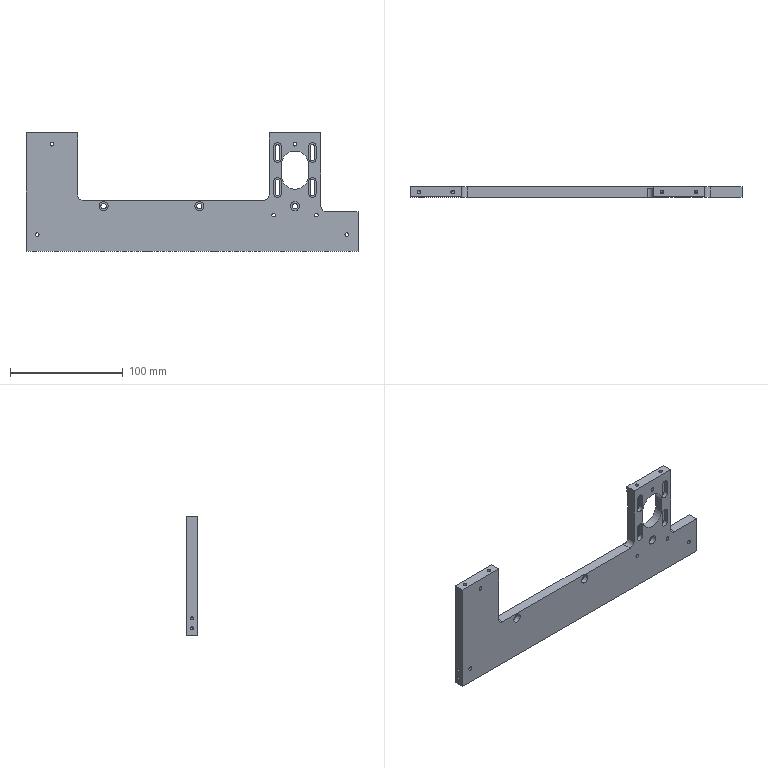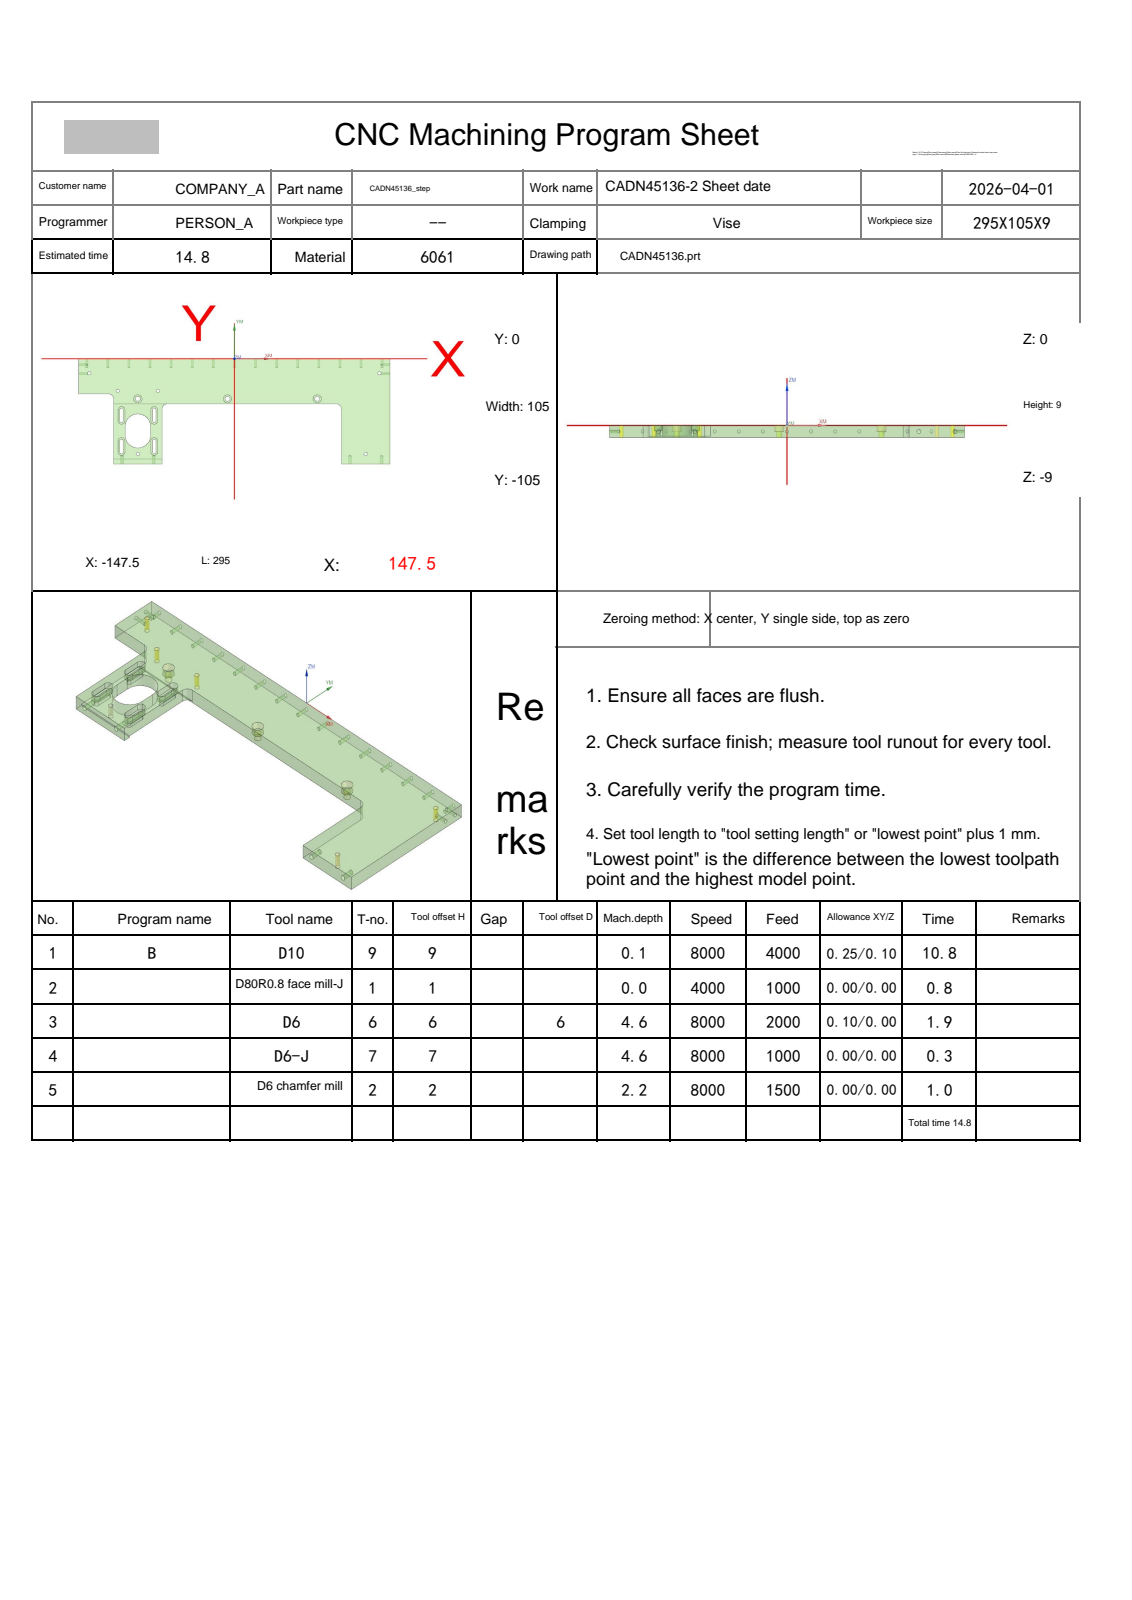NC program | NX | posted by the shop | part box 295 x 9 x 105 mm
Lines 2214 to 3343 of 3343:
N2 T01 M06
(D80R0.8 face mill-J  D=80. R=0.8 H=01 ce=0.00 di=0.00)
G00 G90 G54 X-199.499 Y-24.001 M03 S4000
G43 H01 Z20.
M08
Z2.
G01 Z0.0 F1000.
X-187.499
X179.503
G02 X187.499 Y-31.997 I-.004 J-8.
G01 Y-65.639
G02 X179.499 Y-73.639 I-8. J0.0
G01 X-187.499
X-199.499
Z2.
G00 Z20.
G91 G28 Z0.0
M05
M09
G91 G28 Z0.0
M01
N3 T06 M06
(D6  D=6. R=0. H=06 ce=0.10 di=0.00)
G00 G90 G54 X-91.5 Y-40. M03 S8000
G43 H06 Z20.
M08
Z.3
G41 D06
G01 X-91.505 Y-39.9 F2000.
G03 X-91.947 Y-39.547 I-.442 J-.1
X-92.4 Y-40. I0.0 J-.453
X-92.4 Y-40. Z-.05 I.9 J0.0
X-92.4 Y-40. Z-.4 I.9 J0.0
X-92.4 Y-40. Z-.75 I.9 J0.0
X-92.4 Y-40. Z-1.1 I.9 J0.0
X-92.4 Y-40. Z-1.45 I.9 J0.0
X-92.4 Y-40. Z-1.8 I.9 J0.0
X-92.4 Y-40. Z-2.15 I.9 J0.0
X-92.4 Y-40. Z-2.5 I.9 J0.0
X-92.4 Y-40. Z-2.85 I.9 J0.0
X-92.4 Y-40. Z-3.2 I.9 J0.0
X-92.4 Y-40. Z-3.55 I.9 J0.0
X-92.4 Y-40. Z-3.9 I.9 J0.0
X-92.4 Y-40. Z-4.25 I.9 J0.0
X-92.4 Y-40. Z-4.6 I.9 J0.0
X-91.5 Y-40.9 I.9 J0.0
X-90.6 Y-40. I0.0 J.9
X-91.5 Y-39.1 I-.9 J0.0
X-92.4 Y-40. I0.0 J-.9
X-91.947 Y-40.453 I.453 J0.0
X-91.505 Y-40.1 I0.0 J.453
G01 G40 X-91.5 Y-40.
G00 Z20.
X-6.5
Z.3
G41 D06
G01 X-6.505 Y-39.9
G03 X-6.947 Y-39.547 I-.442 J-.1
X-7.4 Y-40. I0.0 J-.453
X-7.4 Y-40. Z-.05 I.9 J0.0
X-7.4 Y-40. Z-.4 I.9 J0.0
X-7.4 Y-40. Z-.75 I.9 J0.0
X-7.4 Y-40. Z-1.1 I.9 J0.0
X-7.4 Y-40. Z-1.45 I.9 J0.0
X-7.4 Y-40. Z-1.8 I.9 J0.0
X-7.4 Y-40. Z-2.15 I.9 J0.0
X-7.4 Y-40. Z-2.5 I.9 J0.0
X-7.4 Y-40. Z-2.85 I.9 J0.0
X-7.4 Y-40. Z-3.2 I.9 J0.0
X-7.4 Y-40. Z-3.55 I.9 J0.0
X-7.4 Y-40. Z-3.9 I.9 J0.0
X-7.4 Y-40. Z-4.25 I.9 J0.0
X-7.4 Y-40. Z-4.6 I.9 J0.0
X-6.5 Y-40.9 I.9 J0.0
X-5.6 Y-40. I0.0 J.9
X-6.5 Y-39.1 I-.9 J0.0
X-7.4 Y-40. I0.0 J-.9
X-6.947 Y-40.453 I.453 J0.0
X-6.505 Y-40.1 I0.0 J.453
G01 G40 X-6.5 Y-40.
G00 Z20.
X78.5
Z.3
G41 D06
G01 X78.495 Y-39.9
G03 X78.053 Y-39.547 I-.442 J-.1
X77.6 Y-40. I0.0 J-.453
X77.6 Y-40. Z-.05 I.9 J0.0
X77.6 Y-40. Z-.4 I.9 J0.0
X77.6 Y-40. Z-.75 I.9 J0.0
X77.6 Y-40. Z-1.1 I.9 J0.0
X77.6 Y-40. Z-1.45 I.9 J0.0
X77.6 Y-40. Z-1.8 I.9 J0.0
X77.6 Y-40. Z-2.15 I.9 J0.0
X77.6 Y-40. Z-2.5 I.9 J0.0
X77.6 Y-40. Z-2.85 I.9 J0.0
X77.6 Y-40. Z-3.2 I.9 J0.0
X77.6 Y-40. Z-3.55 I.9 J0.0
X77.6 Y-40. Z-3.9 I.9 J0.0
X77.6 Y-40. Z-4.25 I.9 J0.0
X77.6 Y-40. Z-4.6 I.9 J0.0
X78.5 Y-40.9 I.9 J0.0
X79.4 Y-40. I0.0 J.9
X78.5 Y-39.1 I-.9 J0.0
X77.6 Y-40. I0.0 J-.9
X78.053 Y-40.453 I.453 J0.0
X78.495 Y-40.1 I0.0 J.453
G01 G40 X78.5 Y-40.
G00 Z20.
G00 G90 X-75.85 Y-57.849 M03 S8000
Z20.
Z1.
G01 Y-50.851 Z.633 F1200.
X-75.901 Y-50.8 Z.629
X-76. Z.624
X-76.099 Z.619
X-76.15 Y-50.851 Z.615
Y-62.149 Z.023
X-76.099 Y-62.2 Z.019
X-76. Z.014
X-75.901 Z.009
X-75.85 Y-62.149 Z.005
Y-62.05 Z0.0
Y-50.95 Z-.094
G03 X-76. Y-50.8 Z-.096 I-.15 J0.0
X-76.15 Y-50.95 Z-.098 I0.0 J-.15
G01 Y-62.05 Z-.191
G03 X-76. Y-62.2 Z-.193 I.15 J0.0
X-75.85 Y-62.05 Z-.195 I0.0 J.15
G01 Y-50.95 Z-.289
G03 X-76. Y-50.8 Z-.291 I-.15 J0.0
X-76.15 Y-50.95 Z-.293 I0.0 J-.15
G01 Y-62.05 Z-.386
G03 X-76. Y-62.2 Z-.388 I.15 J0.0
X-75.85 Y-62.05 Z-.39 I0.0 J.15
G01 Y-50.95 Z-.484
G03 X-76. Y-50.8 Z-.486 I-.15 J0.0
X-76.15 Y-50.95 Z-.488 I0.0 J-.15
G01 Y-62.05 Z-.581
G03 X-76. Y-62.2 Z-.583 I.15 J0.0
X-75.85 Y-62.05 Z-.585 I0.0 J.15
G01 Y-50.95 Z-.679
G03 X-76. Y-50.8 Z-.681 I-.15 J0.0
X-76.15 Y-50.95 Z-.683 I0.0 J-.15
G01 Y-62.05 Z-.776
G03 X-76. Y-62.2 Z-.778 I.15 J0.0
X-75.85 Y-62.05 Z-.78 I0.0 J.15
G01 Y-50.95 Z-.874
G03 X-76. Y-50.8 Z-.876 I-.15 J0.0
X-76.15 Y-50.95 Z-.878 I0.0 J-.15
G01 Y-62.05 Z-.971
G03 X-76. Y-62.2 Z-.973 I.15 J0.0
X-75.85 Y-62.05 Z-.975 I0.0 J.15
G01 Y-50.95 Z-1.069
G03 X-76. Y-50.8 Z-1.071 I-.15 J0.0
X-76.15 Y-50.95 Z-1.073 I0.0 J-.15
G01 Y-62.05 Z-1.166
G03 X-76. Y-62.2 Z-1.168 I.15 J0.0
X-75.85 Y-62.05 Z-1.17 I0.0 J.15
G01 Y-50.95 Z-1.264
G03 X-76. Y-50.8 Z-1.266 I-.15 J0.0
X-76.15 Y-50.95 Z-1.268 I0.0 J-.15
G01 Y-62.05 Z-1.361
G03 X-76. Y-62.2 Z-1.363 I.15 J0.0
X-75.85 Y-62.05 Z-1.365 I0.0 J.15
G01 Y-50.95 Z-1.459
G03 X-76. Y-50.8 Z-1.461 I-.15 J0.0
X-76.15 Y-50.95 Z-1.463 I0.0 J-.15
G01 Y-62.05 Z-1.556
G03 X-76. Y-62.2 Z-1.558 I.15 J0.0
X-75.85 Y-62.05 Z-1.56 I0.0 J.15
G01 Y-50.95 Z-1.654
G03 X-76. Y-50.8 Z-1.656 I-.15 J0.0
X-76.15 Y-50.95 Z-1.658 I0.0 J-.15
G01 Y-62.05 Z-1.751
G03 X-76. Y-62.2 Z-1.753 I.15 J0.0
X-75.85 Y-62.05 Z-1.755 I0.0 J.15
G01 Y-50.95 Z-1.849
G03 X-76. Y-50.8 Z-1.851 I-.15 J0.0
X-76.15 Y-50.95 Z-1.853 I0.0 J-.15
G01 Y-62.05 Z-1.946
G03 X-76. Y-62.2 Z-1.948 I.15 J0.0
X-75.85 Y-62.05 Z-1.95 I0.0 J.15
G01 Y-50.95 Z-2.044
G03 X-76. Y-50.8 Z-2.046 I-.15 J0.0
X-76.15 Y-50.95 Z-2.048 I0.0 J-.15
G01 Y-62.05 Z-2.141
G03 X-76. Y-62.2 Z-2.143 I.15 J0.0
X-75.85 Y-62.05 Z-2.145 I0.0 J.15
G01 Y-50.95 Z-2.239
G03 X-76. Y-50.8 Z-2.241 I-.15 J0.0
X-76.15 Y-50.95 Z-2.243 I0.0 J-.15
G01 Y-62.05 Z-2.336
G03 X-76. Y-62.2 Z-2.338 I.15 J0.0
X-75.85 Y-62.05 Z-2.34 I0.0 J.15
G01 Y-50.95 Z-2.434
G03 X-76. Y-50.8 Z-2.436 I-.15 J0.0
X-76.15 Y-50.95 Z-2.438 I0.0 J-.15
G01 Y-62.05 Z-2.531
G03 X-76. Y-62.2 Z-2.533 I.15 J0.0
X-75.85 Y-62.05 Z-2.535 I0.0 J.15
G01 Y-50.95 Z-2.629
G03 X-76. Y-50.8 Z-2.631 I-.15 J0.0
X-76.15 Y-50.95 Z-2.633 I0.0 J-.15
G01 Y-62.05 Z-2.726
G03 X-76. Y-62.2 Z-2.728 I.15 J0.0
X-75.85 Y-62.05 Z-2.73 I0.0 J.15
G01 Y-50.95 Z-2.824
G03 X-76. Y-50.8 Z-2.826 I-.15 J0.0
X-76.15 Y-50.95 Z-2.828 I0.0 J-.15
G01 Y-62.05 Z-2.921
G03 X-76. Y-62.2 Z-2.923 I.15 J0.0
X-75.85 Y-62.05 Z-2.925 I0.0 J.15
G01 Y-50.95 Z-3.019
G03 X-76. Y-50.8 Z-3.021 I-.15 J0.0
X-76.15 Y-50.95 Z-3.023 I0.0 J-.15
G01 Y-62.05 Z-3.116
G03 X-76. Y-62.2 Z-3.118 I.15 J0.0
X-75.85 Y-62.05 Z-3.12 I0.0 J.15
G01 Y-50.95 Z-3.214
G03 X-76. Y-50.8 Z-3.216 I-.15 J0.0
X-76.15 Y-50.95 Z-3.218 I0.0 J-.15
G01 Y-62.05 Z-3.311
G03 X-76. Y-62.2 Z-3.313 I.15 J0.0
X-75.85 Y-62.05 Z-3.315 I0.0 J.15
G01 Y-50.95 Z-3.409
G03 X-76. Y-50.8 Z-3.411 I-.15 J0.0
X-76.15 Y-50.95 Z-3.413 I0.0 J-.15
G01 Y-62.05 Z-3.506
G03 X-76. Y-62.2 Z-3.508 I.15 J0.0
X-75.85 Y-62.05 Z-3.51 I0.0 J.15
G01 Y-50.95 Z-3.604
G03 X-76. Y-50.8 Z-3.606 I-.15 J0.0
X-76.15 Y-50.95 Z-3.608 I0.0 J-.15
G01 Y-62.05 Z-3.701
G03 X-76. Y-62.2 Z-3.703 I.15 J0.0
X-75.85 Y-62.05 Z-3.705 I0.0 J.15
G01 Y-50.95 Z-3.799
G03 X-76. Y-50.8 Z-3.801 I-.15 J0.0
X-76.15 Y-50.95 Z-3.803 I0.0 J-.15
G01 Y-62.05 Z-3.896
G03 X-76. Y-62.2 Z-3.898 I.15 J0.0
X-75.85 Y-62.05 Z-3.9 I0.0 J.15
G01 Y-50.95
G03 X-76. Y-50.8 I-.15 J0.0
X-76.15 Y-50.95 I0.0 J-.15
G01 Y-62.05
G03 X-76. Y-62.2 I.15 J0.0
X-75.85 Y-62.05 I0.0 J.15
G01 Y-61.65
Z-2.9
G00 Z20.
X-106.85 Y-57.849
Z1.
G01 Y-50.851 Z.633
X-106.901 Y-50.8 Z.629
X-107.099 Z.619
X-107.15 Y-50.851 Z.615
Y-62.149 Z.023
X-107.099 Y-62.2 Z.019
X-106.901 Z.009
X-106.85 Y-62.149 Z.005
Y-62.05 Z0.0
Y-50.95 Z-.094
G03 X-107. Y-50.8 Z-.096 I-.15 J0.0
X-107.15 Y-50.95 Z-.098 I0.0 J-.15
G01 Y-62.05 Z-.191
G03 X-107. Y-62.2 Z-.193 I.15 J0.0
X-106.85 Y-62.05 Z-.195 I0.0 J.15
G01 Y-50.95 Z-.289
G03 X-107. Y-50.8 Z-.291 I-.15 J0.0
X-107.15 Y-50.95 Z-.293 I0.0 J-.15
G01 Y-62.05 Z-.386
G03 X-107. Y-62.2 Z-.388 I.15 J0.0
X-106.85 Y-62.05 Z-.39 I0.0 J.15
G01 Y-50.95 Z-.484
G03 X-107. Y-50.8 Z-.486 I-.15 J0.0
X-107.15 Y-50.95 Z-.488 I0.0 J-.15
G01 Y-62.05 Z-.581
G03 X-107. Y-62.2 Z-.583 I.15 J0.0
X-106.85 Y-62.05 Z-.585 I0.0 J.15
G01 Y-50.95 Z-.679
G03 X-107. Y-50.8 Z-.681 I-.15 J0.0
X-107.15 Y-50.95 Z-.683 I0.0 J-.15
G01 Y-62.05 Z-.776
G03 X-107. Y-62.2 Z-.778 I.15 J0.0
X-106.85 Y-62.05 Z-.78 I0.0 J.15
G01 Y-50.95 Z-.874
G03 X-107. Y-50.8 Z-.876 I-.15 J0.0
X-107.15 Y-50.95 Z-.878 I0.0 J-.15
G01 Y-62.05 Z-.971
G03 X-107. Y-62.2 Z-.973 I.15 J0.0
X-106.85 Y-62.05 Z-.975 I0.0 J.15
G01 Y-50.95 Z-1.069
G03 X-107. Y-50.8 Z-1.071 I-.15 J0.0
X-107.15 Y-50.95 Z-1.073 I0.0 J-.15
G01 Y-62.05 Z-1.166
G03 X-107. Y-62.2 Z-1.168 I.15 J0.0
X-106.85 Y-62.05 Z-1.17 I0.0 J.15
G01 Y-50.95 Z-1.264
G03 X-107. Y-50.8 Z-1.266 I-.15 J0.0
X-107.15 Y-50.95 Z-1.268 I0.0 J-.15
G01 Y-62.05 Z-1.361
G03 X-107. Y-62.2 Z-1.363 I.15 J0.0
X-106.85 Y-62.05 Z-1.365 I0.0 J.15
G01 Y-50.95 Z-1.459
G03 X-107. Y-50.8 Z-1.461 I-.15 J0.0
X-107.15 Y-50.95 Z-1.463 I0.0 J-.15
G01 Y-62.05 Z-1.556
G03 X-107. Y-62.2 Z-1.558 I.15 J0.0
X-106.85 Y-62.05 Z-1.56 I0.0 J.15
G01 Y-50.95 Z-1.654
G03 X-107. Y-50.8 Z-1.656 I-.15 J0.0
X-107.15 Y-50.95 Z-1.658 I0.0 J-.15
G01 Y-62.05 Z-1.751
G03 X-107. Y-62.2 Z-1.753 I.15 J0.0
X-106.85 Y-62.05 Z-1.755 I0.0 J.15
G01 Y-50.95 Z-1.849
G03 X-107. Y-50.8 Z-1.851 I-.15 J0.0
X-107.15 Y-50.95 Z-1.853 I0.0 J-.15
G01 Y-62.05 Z-1.946
G03 X-107. Y-62.2 Z-1.948 I.15 J0.0
X-106.85 Y-62.05 Z-1.95 I0.0 J.15
G01 Y-50.95 Z-2.044
G03 X-107. Y-50.8 Z-2.046 I-.15 J0.0
X-107.15 Y-50.95 Z-2.048 I0.0 J-.15
G01 Y-62.05 Z-2.141
G03 X-107. Y-62.2 Z-2.143 I.15 J0.0
X-106.85 Y-62.05 Z-2.145 I0.0 J.15
G01 Y-50.95 Z-2.239
G03 X-107. Y-50.8 Z-2.241 I-.15 J0.0
X-107.15 Y-50.95 Z-2.243 I0.0 J-.15
G01 Y-62.05 Z-2.336
G03 X-107. Y-62.2 Z-2.338 I.15 J0.0
X-106.85 Y-62.05 Z-2.34 I0.0 J.15
G01 Y-50.95 Z-2.434
G03 X-107. Y-50.8 Z-2.436 I-.15 J0.0
X-107.15 Y-50.95 Z-2.438 I0.0 J-.15
G01 Y-62.05 Z-2.531
G03 X-107. Y-62.2 Z-2.533 I.15 J0.0
X-106.85 Y-62.05 Z-2.535 I0.0 J.15
G01 Y-50.95 Z-2.629
G03 X-107. Y-50.8 Z-2.631 I-.15 J0.0
X-107.15 Y-50.95 Z-2.633 I0.0 J-.15
G01 Y-62.05 Z-2.726
G03 X-107. Y-62.2 Z-2.728 I.15 J0.0
X-106.85 Y-62.05 Z-2.73 I0.0 J.15
G01 Y-50.95 Z-2.824
G03 X-107. Y-50.8 Z-2.826 I-.15 J0.0
X-107.15 Y-50.95 Z-2.828 I0.0 J-.15
G01 Y-62.05 Z-2.921
G03 X-107. Y-62.2 Z-2.923 I.15 J0.0
X-106.85 Y-62.05 Z-2.925 I0.0 J.15
G01 Y-50.95 Z-3.019
G03 X-107. Y-50.8 Z-3.021 I-.15 J0.0
X-107.15 Y-50.95 Z-3.023 I0.0 J-.15
G01 Y-62.05 Z-3.116
G03 X-107. Y-62.2 Z-3.118 I.15 J0.0
X-106.85 Y-62.05 Z-3.12 I0.0 J.15
G01 Y-50.95 Z-3.214
G03 X-107. Y-50.8 Z-3.216 I-.15 J0.0
X-107.15 Y-50.95 Z-3.218 I0.0 J-.15
G01 Y-62.05 Z-3.311
G03 X-107. Y-62.2 Z-3.313 I.15 J0.0
X-106.85 Y-62.05 Z-3.315 I0.0 J.15
G01 Y-50.95 Z-3.409
G03 X-107. Y-50.8 Z-3.411 I-.15 J0.0
X-107.15 Y-50.95 Z-3.413 I0.0 J-.15
G01 Y-62.05 Z-3.506
G03 X-107. Y-62.2 Z-3.508 I.15 J0.0
X-106.85 Y-62.05 Z-3.51 I0.0 J.15
G01 Y-50.95 Z-3.604
G03 X-107. Y-50.8 Z-3.606 I-.15 J0.0
X-107.15 Y-50.95 Z-3.608 I0.0 J-.15
G01 Y-62.05 Z-3.701
G03 X-107. Y-62.2 Z-3.703 I.15 J0.0
X-106.85 Y-62.05 Z-3.705 I0.0 J.15
G01 Y-50.95 Z-3.799
G03 X-107. Y-50.8 Z-3.801 I-.15 J0.0
X-107.15 Y-50.95 Z-3.803 I0.0 J-.15
G01 Y-62.05 Z-3.896
G03 X-107. Y-62.2 Z-3.898 I.15 J0.0
X-106.85 Y-62.05 Z-3.9 I0.0 J.15
G01 Y-50.95
G03 X-107. Y-50.8 I-.15 J0.0
X-107.15 Y-50.95 I0.0 J-.15
G01 Y-62.05
G03 X-107. Y-62.2 I.15 J0.0
X-106.85 Y-62.05 I0.0 J.15
G01 Y-61.65
Z-2.9
G00 Z20.
Y-88.849
Z1.
G01 Y-81.95 Z.638
Y-81.851 Z.633
X-106.901 Y-81.8 Z.629
X-107. Z.624
X-107.099 Z.619
X-107.15 Y-81.851 Z.615
Y-93.149 Z.023
X-107.099 Y-93.2 Z.019
X-106.901 Z.009
X-106.85 Y-93.149 Z.005
Y-93.05 Z0.0
Y-81.95 Z-.094
G03 X-107. Y-81.8 Z-.096 I-.15 J0.0
X-107.15 Y-81.95 Z-.098 I0.0 J-.15
G01 Y-93.05 Z-.191
G03 X-107. Y-93.2 Z-.193 I.15 J0.0
X-106.85 Y-93.05 Z-.195 I0.0 J.15
G01 Y-81.95 Z-.289
G03 X-107. Y-81.8 Z-.291 I-.15 J0.0
X-107.15 Y-81.95 Z-.293 I0.0 J-.15
G01 Y-93.05 Z-.386
G03 X-107. Y-93.2 Z-.388 I.15 J0.0
X-106.85 Y-93.05 Z-.39 I0.0 J.15
G01 Y-81.95 Z-.484
G03 X-107. Y-81.8 Z-.486 I-.15 J0.0
X-107.15 Y-81.95 Z-.488 I0.0 J-.15
G01 Y-93.05 Z-.581
G03 X-107. Y-93.2 Z-.583 I.15 J0.0
X-106.85 Y-93.05 Z-.585 I0.0 J.15
G01 Y-81.95 Z-.679
G03 X-107. Y-81.8 Z-.681 I-.15 J0.0
X-107.15 Y-81.95 Z-.683 I0.0 J-.15
G01 Y-93.05 Z-.776
G03 X-107. Y-93.2 Z-.778 I.15 J0.0
X-106.85 Y-93.05 Z-.78 I0.0 J.15
G01 Y-81.95 Z-.874
G03 X-107. Y-81.8 Z-.876 I-.15 J0.0
X-107.15 Y-81.95 Z-.878 I0.0 J-.15
G01 Y-93.05 Z-.971
G03 X-107. Y-93.2 Z-.973 I.15 J0.0
X-106.85 Y-93.05 Z-.975 I0.0 J.15
G01 Y-81.95 Z-1.069
G03 X-107. Y-81.8 Z-1.071 I-.15 J0.0
X-107.15 Y-81.95 Z-1.073 I0.0 J-.15
G01 Y-93.05 Z-1.166
G03 X-107. Y-93.2 Z-1.168 I.15 J0.0
X-106.85 Y-93.05 Z-1.17 I0.0 J.15
G01 Y-81.95 Z-1.264
G03 X-107. Y-81.8 Z-1.266 I-.15 J0.0
X-107.15 Y-81.95 Z-1.268 I0.0 J-.15
G01 Y-93.05 Z-1.361
G03 X-107. Y-93.2 Z-1.363 I.15 J0.0
X-106.85 Y-93.05 Z-1.365 I0.0 J.15
G01 Y-81.95 Z-1.459
G03 X-107. Y-81.8 Z-1.461 I-.15 J0.0
X-107.15 Y-81.95 Z-1.463 I0.0 J-.15
G01 Y-93.05 Z-1.556
G03 X-107. Y-93.2 Z-1.558 I.15 J0.0
X-106.85 Y-93.05 Z-1.56 I0.0 J.15
G01 Y-81.95 Z-1.654
G03 X-107. Y-81.8 Z-1.656 I-.15 J0.0
X-107.15 Y-81.95 Z-1.658 I0.0 J-.15
G01 Y-93.05 Z-1.751
G03 X-107. Y-93.2 Z-1.753 I.15 J0.0
X-106.85 Y-93.05 Z-1.755 I0.0 J.15
G01 Y-81.95 Z-1.849
G03 X-107. Y-81.8 Z-1.851 I-.15 J0.0
X-107.15 Y-81.95 Z-1.853 I0.0 J-.15
G01 Y-93.05 Z-1.946
G03 X-107. Y-93.2 Z-1.948 I.15 J0.0
X-106.85 Y-93.05 Z-1.95 I0.0 J.15
G01 Y-81.95 Z-2.044
G03 X-107. Y-81.8 Z-2.046 I-.15 J0.0
X-107.15 Y-81.95 Z-2.048 I0.0 J-.15
G01 Y-93.05 Z-2.141
G03 X-107. Y-93.2 Z-2.143 I.15 J0.0
X-106.85 Y-93.05 Z-2.145 I0.0 J.15
G01 Y-81.95 Z-2.239
G03 X-107. Y-81.8 Z-2.241 I-.15 J0.0
X-107.15 Y-81.95 Z-2.243 I0.0 J-.15
G01 Y-93.05 Z-2.336
G03 X-107. Y-93.2 Z-2.338 I.15 J0.0
X-106.85 Y-93.05 Z-2.34 I0.0 J.15
G01 Y-81.95 Z-2.434
G03 X-107. Y-81.8 Z-2.436 I-.15 J0.0
X-107.15 Y-81.95 Z-2.438 I0.0 J-.15
G01 Y-93.05 Z-2.531
G03 X-107. Y-93.2 Z-2.533 I.15 J0.0
X-106.85 Y-93.05 Z-2.535 I0.0 J.15
G01 Y-81.95 Z-2.629
G03 X-107. Y-81.8 Z-2.631 I-.15 J0.0
X-107.15 Y-81.95 Z-2.633 I0.0 J-.15
G01 Y-93.05 Z-2.726
G03 X-107. Y-93.2 Z-2.728 I.15 J0.0
X-106.85 Y-93.05 Z-2.73 I0.0 J.15
G01 Y-81.95 Z-2.824
G03 X-107. Y-81.8 Z-2.826 I-.15 J0.0
X-107.15 Y-81.95 Z-2.828 I0.0 J-.15
G01 Y-93.05 Z-2.921
G03 X-107. Y-93.2 Z-2.923 I.15 J0.0
X-106.85 Y-93.05 Z-2.925 I0.0 J.15
G01 Y-81.95 Z-3.019
G03 X-107. Y-81.8 Z-3.021 I-.15 J0.0
X-107.15 Y-81.95 Z-3.023 I0.0 J-.15
G01 Y-93.05 Z-3.116
G03 X-107. Y-93.2 Z-3.118 I.15 J0.0
X-106.85 Y-93.05 Z-3.12 I0.0 J.15
G01 Y-81.95 Z-3.214
G03 X-107. Y-81.8 Z-3.216 I-.15 J0.0
X-107.15 Y-81.95 Z-3.218 I0.0 J-.15
G01 Y-93.05 Z-3.311
G03 X-107. Y-93.2 Z-3.313 I.15 J0.0
X-106.85 Y-93.05 Z-3.315 I0.0 J.15
G01 Y-81.95 Z-3.409
G03 X-107. Y-81.8 Z-3.411 I-.15 J0.0
X-107.15 Y-81.95 Z-3.413 I0.0 J-.15
G01 Y-93.05 Z-3.506
G03 X-107. Y-93.2 Z-3.508 I.15 J0.0
X-106.85 Y-93.05 Z-3.51 I0.0 J.15
G01 Y-81.95 Z-3.604
G03 X-107. Y-81.8 Z-3.606 I-.15 J0.0
X-107.15 Y-81.95 Z-3.608 I0.0 J-.15
G01 Y-93.05 Z-3.701
G03 X-107. Y-93.2 Z-3.703 I.15 J0.0
X-106.85 Y-93.05 Z-3.705 I0.0 J.15
G01 Y-81.95 Z-3.799
G03 X-107. Y-81.8 Z-3.801 I-.15 J0.0
X-107.15 Y-81.95 Z-3.803 I0.0 J-.15
G01 Y-93.05 Z-3.896
G03 X-107. Y-93.2 Z-3.898 I.15 J0.0
X-106.85 Y-93.05 Z-3.9 I0.0 J.15
G01 Y-81.95
G03 X-107. Y-81.8 I-.15 J0.0
X-107.15 Y-81.95 I0.0 J-.15
G01 Y-93.05
G03 X-107. Y-93.2 I.15 J0.0
X-106.85 Y-93.05 I0.0 J.15
G01 Y-92.65
Z-2.9
G00 Z20.
X-76.15 Y-86.151
Z1.
G01 Y-93.05 Z.638
Y-93.149 Z.633
X-76.099 Y-93.2 Z.629
X-75.901 Z.619
X-75.85 Y-93.149 Z.615
Y-81.851 Z.023
X-75.901 Y-81.8 Z.019
X-76. Z.014
X-76.099 Z.009
X-76.15 Y-81.851 Z.005
Y-81.95 Z0.0
Y-93.05 Z-.094
G03 X-76. Y-93.2 Z-.096 I.15 J0.0
X-75.85 Y-93.05 Z-.098 I0.0 J.15
G01 Y-81.95 Z-.191
G03 X-76. Y-81.8 Z-.193 I-.15 J0.0
X-76.15 Y-81.95 Z-.195 I0.0 J-.15
G01 Y-93.05 Z-.289
G03 X-76. Y-93.2 Z-.291 I.15 J0.0
X-75.85 Y-93.05 Z-.293 I0.0 J.15
G01 Y-81.95 Z-.386
G03 X-76. Y-81.8 Z-.388 I-.15 J0.0
X-76.15 Y-81.95 Z-.39 I0.0 J-.15
G01 Y-93.05 Z-.484
G03 X-76. Y-93.2 Z-.486 I.15 J0.0
X-75.85 Y-93.05 Z-.488 I0.0 J.15
G01 Y-81.95 Z-.581
G03 X-76. Y-81.8 Z-.583 I-.15 J0.0
X-76.15 Y-81.95 Z-.585 I0.0 J-.15
G01 Y-93.05 Z-.679
G03 X-76. Y-93.2 Z-.681 I.15 J0.0
X-75.85 Y-93.05 Z-.683 I0.0 J.15
G01 Y-81.95 Z-.776
G03 X-76. Y-81.8 Z-.778 I-.15 J0.0
X-76.15 Y-81.95 Z-.78 I0.0 J-.15
G01 Y-93.05 Z-.874
G03 X-76. Y-93.2 Z-.876 I.15 J0.0
X-75.85 Y-93.05 Z-.878 I0.0 J.15
G01 Y-81.95 Z-.971
G03 X-76. Y-81.8 Z-.973 I-.15 J0.0
X-76.15 Y-81.95 Z-.975 I0.0 J-.15
G01 Y-93.05 Z-1.069
G03 X-76. Y-93.2 Z-1.071 I.15 J0.0
X-75.85 Y-93.05 Z-1.073 I0.0 J.15
G01 Y-81.95 Z-1.166
G03 X-76. Y-81.8 Z-1.168 I-.15 J0.0
X-76.15 Y-81.95 Z-1.17 I0.0 J-.15
G01 Y-93.05 Z-1.264
G03 X-76. Y-93.2 Z-1.266 I.15 J0.0
X-75.85 Y-93.05 Z-1.268 I0.0 J.15
G01 Y-81.95 Z-1.361
G03 X-76. Y-81.8 Z-1.363 I-.15 J0.0
X-76.15 Y-81.95 Z-1.365 I0.0 J-.15
G01 Y-93.05 Z-1.459
G03 X-76. Y-93.2 Z-1.461 I.15 J0.0
X-75.85 Y-93.05 Z-1.463 I0.0 J.15
G01 Y-81.95 Z-1.556
G03 X-76. Y-81.8 Z-1.558 I-.15 J0.0
X-76.15 Y-81.95 Z-1.56 I0.0 J-.15
G01 Y-93.05 Z-1.654
G03 X-76. Y-93.2 Z-1.656 I.15 J0.0
X-75.85 Y-93.05 Z-1.658 I0.0 J.15
G01 Y-81.95 Z-1.751
G03 X-76. Y-81.8 Z-1.753 I-.15 J0.0
X-76.15 Y-81.95 Z-1.755 I0.0 J-.15
G01 Y-93.05 Z-1.849
G03 X-76. Y-93.2 Z-1.851 I.15 J0.0
X-75.85 Y-93.05 Z-1.853 I0.0 J.15
G01 Y-81.95 Z-1.946
G03 X-76. Y-81.8 Z-1.948 I-.15 J0.0
X-76.15 Y-81.95 Z-1.95 I0.0 J-.15
G01 Y-93.05 Z-2.044
G03 X-76. Y-93.2 Z-2.046 I.15 J0.0
X-75.85 Y-93.05 Z-2.048 I0.0 J.15
G01 Y-81.95 Z-2.141
G03 X-76. Y-81.8 Z-2.143 I-.15 J0.0
X-76.15 Y-81.95 Z-2.145 I0.0 J-.15
G01 Y-93.05 Z-2.239
G03 X-76. Y-93.2 Z-2.241 I.15 J0.0
X-75.85 Y-93.05 Z-2.243 I0.0 J.15
G01 Y-81.95 Z-2.336
G03 X-76. Y-81.8 Z-2.338 I-.15 J0.0
X-76.15 Y-81.95 Z-2.34 I0.0 J-.15
G01 Y-93.05 Z-2.434
G03 X-76. Y-93.2 Z-2.436 I.15 J0.0
X-75.85 Y-93.05 Z-2.438 I0.0 J.15
G01 Y-81.95 Z-2.531
G03 X-76. Y-81.8 Z-2.533 I-.15 J0.0
X-76.15 Y-81.95 Z-2.535 I0.0 J-.15
G01 Y-93.05 Z-2.629
G03 X-76. Y-93.2 Z-2.631 I.15 J0.0
X-75.85 Y-93.05 Z-2.633 I0.0 J.15
G01 Y-81.95 Z-2.726
G03 X-76. Y-81.8 Z-2.728 I-.15 J0.0
X-76.15 Y-81.95 Z-2.73 I0.0 J-.15
G01 Y-93.05 Z-2.824
G03 X-76. Y-93.2 Z-2.826 I.15 J0.0
X-75.85 Y-93.05 Z-2.828 I0.0 J.15
G01 Y-81.95 Z-2.921
G03 X-76. Y-81.8 Z-2.923 I-.15 J0.0
X-76.15 Y-81.95 Z-2.925 I0.0 J-.15
G01 Y-93.05 Z-3.019
G03 X-76. Y-93.2 Z-3.021 I.15 J0.0
X-75.85 Y-93.05 Z-3.023 I0.0 J.15
G01 Y-81.95 Z-3.116
G03 X-76. Y-81.8 Z-3.118 I-.15 J0.0
X-76.15 Y-81.95 Z-3.12 I0.0 J-.15
G01 Y-93.05 Z-3.214
G03 X-76. Y-93.2 Z-3.216 I.15 J0.0
X-75.85 Y-93.05 Z-3.218 I0.0 J.15
G01 Y-81.95 Z-3.311
G03 X-76. Y-81.8 Z-3.313 I-.15 J0.0
X-76.15 Y-81.95 Z-3.315 I0.0 J-.15
G01 Y-93.05 Z-3.409
G03 X-76. Y-93.2 Z-3.411 I.15 J0.0
X-75.85 Y-93.05 Z-3.413 I0.0 J.15
G01 Y-81.95 Z-3.506
G03 X-76. Y-81.8 Z-3.508 I-.15 J0.0
X-76.15 Y-81.95 Z-3.51 I0.0 J-.15
G01 Y-93.05 Z-3.604
G03 X-76. Y-93.2 Z-3.606 I.15 J0.0
X-75.85 Y-93.05 Z-3.608 I0.0 J.15
G01 Y-81.95 Z-3.701
G03 X-76. Y-81.8 Z-3.703 I-.15 J0.0
X-76.15 Y-81.95 Z-3.705 I0.0 J-.15
G01 Y-93.05 Z-3.799
G03 X-76. Y-93.2 Z-3.801 I.15 J0.0
X-75.85 Y-93.05 Z-3.803 I0.0 J.15
G01 Y-81.95 Z-3.896
G03 X-76. Y-81.8 Z-3.898 I-.15 J0.0
X-76.15 Y-81.95 Z-3.9 I0.0 J-.15
G01 Y-93.05
G03 X-76. Y-93.2 I.15 J0.0
X-75.85 Y-93.05 I0.0 J.15
G01 Y-81.95
G03 X-76. Y-81.8 I-.15 J0.0
X-76.15 Y-81.95 I0.0 J-.15
G01 Y-82.35
Z-2.9
G00 Z20.
G91 G28 Z0.0
M05
M09
G91 G28 Z0.0
M01
N4 T07 M06
(D6-J  D=6. R=0. H=07 ce=0.00 di=0.00)
G00 G90 G54 X-91.5 Y-40. M03 S8000
G43 H07 Z20.
M08
Z-4.6
G01 X-92.029 Y-39.718 F600.
X-92.18 Y-39.68
G03 X-92.5 Y-40. I0.0 J-.32
X-91.5 Y-41. I1. J0.0
X-90.5 Y-40. I0.0 J1.
X-91.5 Y-39. I-1. J0.0
X-92.5 Y-40. I0.0 J-1.
X-92.378 Y-40.479 I1. J0.0
X-92.097 Y-40.646 I.281 J.153
X-91.829 Y-40.502 I0.0 J.32
G01 X-91.5 Y-40.
G00 Z20.
X-6.5
Z-4.6
G01 X-7.029 Y-39.718
X-7.18 Y-39.68
G03 X-7.5 Y-40. I0.0 J-.32
X-6.5 Y-41. I1. J0.0
X-5.5 Y-40. I0.0 J1.
X-6.5 Y-39. I-1. J0.0
X-7.5 Y-40. I0.0 J-1.
X-7.378 Y-40.479 I1. J0.0
X-7.097 Y-40.646 I.281 J.153
X-6.829 Y-40.502 I0.0 J.32
G01 X-6.5 Y-40.
G00 Z20.
X78.5
Z-4.6
G01 X77.971 Y-39.718
X77.82 Y-39.68
G03 X77.5 Y-40. I0.0 J-.32
X78.5 Y-41. I1. J0.0
X79.5 Y-40. I0.0 J1.
X78.5 Y-39. I-1. J0.0
X77.5 Y-40. I0.0 J-1.
X77.622 Y-40.479 I1. J0.0
X77.903 Y-40.646 I.281 J.153
X78.171 Y-40.502 I0.0 J.32
G01 X78.5 Y-40.
G00 Z20.
G00 G90 X-75.822 Y-88.543 M03 S8000
Z12.825
Z1.
G01 Y-81.917 Z-.775 F1000.
X-75.849 Y-81.85 Z-.795
X-75.9 Y-81.799 Z-.814
X-75.967 Y-81.772 Z-.834
X-76.033 Z-.851
X-76.1 Y-81.799 Z-.871
X-76.151 Y-81.85 Z-.89
X-76.178 Y-81.917 Z-.909
Y-93.083 Z-3.901
X-76.151 Y-93.15 Z-3.921
X-76.1 Y-93.201 Z-3.94
X-76.033 Y-93.228 Z-3.96
X-75.967 Z-3.977
X-75.917 Y-93.211 Z-3.991
X-75.891 Y-93.191 Z-4.
G41 D07
X-75.75 Y-93.05
Y-81.95
G03 X-76. Y-81.7 I-.25 J0.0
X-76.25 Y-81.95 I0.0 J-.25
G01 Y-93.05
G03 X-76. Y-93.3 I.25 J0.0
X-75.75 Y-93.05 I0.0 J.25
G01 Y-92.65
G03 X-75.926 Y-92.226 I-.6 J0.0
G01 G40 X-76.067 Y-92.084
Z-3.
G00 Z12.825
X-106.822 Y-88.543
Z1.
G01 Y-81.917 Z-.775
X-106.849 Y-81.85 Z-.795
X-106.9 Y-81.799 Z-.814
X-106.967 Y-81.772 Z-.834
X-107.033 Z-.851
X-107.1 Y-81.799 Z-.871
X-107.151 Y-81.85 Z-.89
X-107.178 Y-81.917 Z-.909
Y-93.083 Z-3.901
X-107.151 Y-93.15 Z-3.921
X-107.1 Y-93.201 Z-3.94
X-107.033 Y-93.228 Z-3.96
X-106.967 Z-3.977
X-106.917 Y-93.211 Z-3.991
X-106.891 Y-93.191 Z-4.
G41 D07
X-106.75 Y-93.05
Y-81.95
G03 X-107. Y-81.7 I-.25 J0.0
X-107.25 Y-81.95 I0.0 J-.25
G01 Y-93.05
G03 X-107. Y-93.3 I.25 J0.0
X-106.75 Y-93.05 I0.0 J.25
G01 Y-92.65
G03 X-106.926 Y-92.226 I-.6 J0.0
G01 G40 X-107.067 Y-92.084
Z-3.
G00 Z12.825
X-107.178 Y-55.457
Z1.
G01 Y-62.083 Z-.775
X-107.151 Y-62.15 Z-.795
X-107.1 Y-62.201 Z-.814
X-107.033 Y-62.228 Z-.834
X-106.967 Z-.851
X-106.9 Y-62.201 Z-.871
X-106.849 Y-62.15 Z-.89
X-106.822 Y-62.083 Z-.909
Y-50.917 Z-3.901
X-106.849 Y-50.85 Z-3.921
X-106.9 Y-50.799 Z-3.94
X-106.967 Y-50.772 Z-3.96
X-107.033 Z-3.977
X-107.083 Y-50.789 Z-3.991
X-107.109 Y-50.809 Z-4.
G41 D07
X-107.25 Y-50.95
Y-62.05
G03 X-107. Y-62.3 I.25 J0.0
X-106.75 Y-62.05 I0.0 J.25
G01 Y-50.95
G03 X-107. Y-50.7 I-.25 J0.0
X-107.25 Y-50.95 I0.0 J-.25
G01 Y-51.35
G03 X-107.074 Y-51.774 I.6 J0.0
G01 G40 X-106.933 Y-51.916
Z-3.
G00 Z12.825
X-75.822 Y-57.543
Z1.
G01 Y-50.917 Z-.775
X-75.849 Y-50.85 Z-.795
X-75.9 Y-50.799 Z-.814
X-75.967 Y-50.772 Z-.834
X-76.033 Z-.851
X-76.1 Y-50.799 Z-.871
X-76.151 Y-50.85 Z-.89
X-76.178 Y-50.917 Z-.909
Y-62.083 Z-3.901
X-76.151 Y-62.15 Z-3.921
X-76.1 Y-62.201 Z-3.94
X-76.033 Y-62.228 Z-3.96
X-75.967 Z-3.977
X-75.917 Y-62.211 Z-3.991
X-75.891 Y-62.191 Z-4.
G41 D07
X-75.75 Y-62.05
Y-50.95
G03 X-76. Y-50.7 I-.25 J0.0
X-76.25 Y-50.95 I0.0 J-.25
G01 Y-62.05
G03 X-76. Y-62.3 I.25 J0.0
X-75.75 Y-62.05 I0.0 J.25
G01 Y-61.65
G03 X-75.926 Y-61.226 I-.6 J0.0
G01 G40 X-76.067 Y-61.084
Z-3.
G00 Z12.825
G91 G28 Z0.0
M05
M09
G91 G28 Z0.0
M01
N5 T02 M06
(D6 chamfer mill  D=6. R=0. H=02 ce=0.00 di=0.00)
G00 G90 G54 X137.5 Y-14.5 M03 S8000
G43 H02 Z20.
M08
G98 G81 X137.5 Y-14.5 Z-2.2 R3. F1000.
X124.5 Y-95.
X-91.5
X-72.5 Y-32.
X-110.5
X-137.5 Y-14.5
G80
G00 Z20.
G00 G90 X-.386 Y1.227 M03 S6500
Z20.
Z.172
G01 Z-1.2 F1500.
G03 X-.1 Y1.027 I1.286 J1.532
G01 X-.054 Y.997
X0.0 Y1.
X147.5
G02 X148.5 Y0.0 I0.0 J-1.
G01 Y-105.
G02 X147.5 Y-106. I-1. J0.0
G01 X101.5
G02 X100.5 Y-105. I0.0 J1.
G01 Y-50.
G03 X96.5 Y-46. I-4. J0.0
G01 X-63.5
G03 X-67.5 Y-50. I0.0 J-4.
G01 Y-105.
G02 X-68.5 Y-106. I-1. J0.0
G01 X-114.5
G02 X-115.5 Y-105. I0.0 J1.
G01 Y-40.
G03 X-119.5 Y-36. I-4. J0.0
G01 X-147.5
G02 X-148.5 Y-35. I0.0 J1.
G01 Y0.0
G02 X-147.5 Y1. I1. J0.0
G01 X0.0
X.054 Y.997
X.1 Y1.027
G03 X.386 Y1.227 I-1. J1.732
G01 Z.172
G00 Z10.
X-137.081 Y-14.006
Z.405
G01 Z-1.2
G03 X-137.397 Y-13.859 I-1. J-1.732
G01 X-137.447 Y-13.838
X-137.5 Y-13.85
G03 X-138.15 Y-14.5 I0.0 J-.65
X-137.5 Y-15.15 I.65 J0.0
X-136.85 Y-14.5 I0.0 J.65
X-137.5 Y-13.85 I-.65 J0.0
G01 X-137.553 Y-13.838
X-137.603 Y-13.859
G03 X-137.919 Y-14.006 I.684 J-1.879
G01 Z.405
G00 Z10.
X-110.081 Y-31.506
Z.405
G01 Z-1.2
G03 X-110.397 Y-31.359 I-1. J-1.732
G01 X-110.447 Y-31.338
X-110.5 Y-31.35
G03 X-111.15 Y-32. I0.0 J-.65
X-110.5 Y-32.65 I.65 J0.0
X-109.85 Y-32. I0.0 J.65
X-110.5 Y-31.35 I-.65 J0.0
G01 X-110.553 Y-31.338
X-110.603 Y-31.359
G03 X-110.919 Y-31.506 I.684 J-1.879
G01 Z.405
G00 Z10.
X-104.977 Y-56.886
Z.172
G01 Z-1.2
G03 X-104.777 Y-56.6 I-1.532 J1.286
G01 X-104.747 Y-56.554
X-104.75 Y-56.5
Y-50.95
G03 X-107. Y-48.7 I-2.25 J0.0
X-109.25 Y-50.95 I0.0 J-2.25
G01 Y-62.05
G03 X-107. Y-64.3 I2.25 J0.0
X-104.75 Y-62.05 I0.0 J2.25
G01 Y-56.5
X-104.747 Y-56.446
X-104.777 Y-56.4
G03 X-104.977 Y-56.114 I-1.732 J-1.
G01 Z.172
G00 Z10.
X-80.727 Y-72.386
Z.172
G01 Z-1.2
G03 X-80.527 Y-72.1 I-1.532 J1.286
G01 X-80.497 Y-72.054
X-80.5 Y-72.
Y-67.
G03 X-91.5 Y-56. I-11. J0.0
X-102.5 Y-67. I0.0 J-11.
G01 Y-77.
G03 X-91.5 Y-88. I11. J0.0
X-80.5 Y-77. I0.0 J11.
G01 Y-72.
X-80.497 Y-71.946
X-80.527 Y-71.9
G03 X-80.727 Y-71.614 I-1.732 J-1.
G01 Z.172
G00 Z10.
X-104.977 Y-87.886
Z.172
G01 Z-1.2
G03 X-104.777 Y-87.6 I-1.532 J1.286
G01 X-104.747 Y-87.554
X-104.75 Y-87.5
Y-81.95
G03 X-107. Y-79.7 I-2.25 J0.0
X-109.25 Y-81.95 I0.0 J-2.25
G01 Y-93.05
G03 X-107. Y-95.3 I2.25 J0.0
X-104.75 Y-93.05 I0.0 J2.25
G01 Y-87.5
X-104.747 Y-87.446
X-104.777 Y-87.4
G03 X-104.977 Y-87.114 I-1.732 J-1.
G01 Z.172
G00 Z10.
X-91.919 Y-95.494
Z.405
G01 Z-1.2
G03 X-91.603 Y-95.641 I1. J1.732
G01 X-91.553 Y-95.662
X-91.5 Y-95.65
G03 X-90.85 Y-95. I0.0 J.65
X-91.5 Y-94.35 I-.65 J0.0
X-92.15 Y-95. I0.0 J-.65
X-91.5 Y-95.65 I.65 J0.0
G01 X-91.447 Y-95.662
X-91.397 Y-95.641
G03 X-91.081 Y-95.494 I-.684 J1.879
G01 Z.405
G00 Z10.
X-73.977 Y-87.886
Z.172
G01 Z-1.2
G03 X-73.777 Y-87.6 I-1.532 J1.286
G01 X-73.747 Y-87.554
X-73.75 Y-87.5
Y-81.95
G03 X-76. Y-79.7 I-2.25 J0.0
X-78.25 Y-81.95 I0.0 J-2.25
G01 Y-93.05
G03 X-76. Y-95.3 I2.25 J0.0
X-73.75 Y-93.05 I0.0 J2.25
G01 Y-87.5
X-73.747 Y-87.446
X-73.777 Y-87.4
G03 X-73.977 Y-87.114 I-1.732 J-1.
G01 Z.172
G00 Z10.
Y-56.886
Z.172
G01 Z-1.2
G03 X-73.777 Y-56.6 I-1.532 J1.286
G01 X-73.747 Y-56.554
X-73.75 Y-56.5
Y-50.95
G03 X-76. Y-48.7 I-2.25 J0.0
X-78.25 Y-50.95 I0.0 J-2.25
G01 Y-62.05
G03 X-76. Y-64.3 I2.25 J0.0
X-73.75 Y-62.05 I0.0 J2.25
G01 Y-56.5
X-73.747 Y-56.446
X-73.777 Y-56.4
G03 X-73.977 Y-56.114 I-1.732 J-1.
G01 Z.172
G00 Z10.
X-91.099 Y-37.197
Z.233
G01 Z-1.2
G03 X-91.398 Y-37.019 I-1.167 J-1.624
G01 X-91.446 Y-36.993
X-91.5 Y-37.
G03 X-94.5 Y-40. I0.0 J-3.
X-91.5 Y-43. I3. J0.0
X-88.5 Y-40. I0.0 J3.
X-91.5 Y-37. I-3. J0.0
G01 X-91.554 Y-36.993
X-91.602 Y-37.019
G03 X-91.901 Y-37.197 I.868 J-1.802
G01 Z.233
G00 Z10.
X-72.081 Y-31.506
Z.405
G01 Z-1.2
G03 X-72.397 Y-31.359 I-1. J-1.732
G01 X-72.447 Y-31.338
X-72.5 Y-31.35
G03 X-73.15 Y-32. I0.0 J-.65
X-72.5 Y-32.65 I.65 J0.0
X-71.85 Y-32. I0.0 J.65
X-72.5 Y-31.35 I-.65 J0.0
G01 X-72.553 Y-31.338
X-72.603 Y-31.359
G03 X-72.919 Y-31.506 I.684 J-1.879
G01 Z.405
G00 Z10.
X-6.099 Y-37.197
Z.233
G01 Z-1.2
G03 X-6.398 Y-37.019 I-1.167 J-1.624
G01 X-6.446 Y-36.993
X-6.5 Y-37.
G03 X-9.5 Y-40. I0.0 J-3.
X-6.5 Y-43. I3. J0.0
X-3.5 Y-40. I0.0 J3.
X-6.5 Y-37. I-3. J0.0
G01 X-6.554 Y-36.993
X-6.602 Y-37.019
G03 X-6.901 Y-37.197 I.868 J-1.802
G01 Z.233
G00 Z10.
X78.901
Z.233
G01 Z-1.2
G03 X78.602 Y-37.019 I-1.167 J-1.624
G01 X78.554 Y-36.993
X78.5 Y-37.
G03 X75.5 Y-40. I0.0 J-3.
X78.5 Y-43. I3. J0.0
X81.5 Y-40. I0.0 J3.
X78.5 Y-37. I-3. J0.0
G01 X78.446 Y-36.993
X78.398 Y-37.019
G03 X78.099 Y-37.197 I.868 J-1.802
G01 Z.233
G00 Z10.
X137.919 Y-14.006
Z.405
G01 Z-1.2
G03 X137.603 Y-13.859 I-1. J-1.732
G01 X137.553 Y-13.838
X137.5 Y-13.85
G03 X136.85 Y-14.5 I0.0 J-.65
X137.5 Y-15.15 I.65 J0.0
X138.15 Y-14.5 I0.0 J.65
X137.5 Y-13.85 I-.65 J0.0
G01 X137.447 Y-13.838
X137.397 Y-13.859
G03 X137.081 Y-14.006 I.684 J-1.879
G01 Z.405
G00 Z10.
X124.081 Y-95.494
Z.405
G01 Z-1.2
G03 X124.397 Y-95.641 I1. J1.732
G01 X124.447 Y-95.662
X124.5 Y-95.65
G03 X125.15 Y-95. I0.0 J.65
X124.5 Y-94.35 I-.65 J0.0
X123.85 Y-95. I0.0 J-.65
X124.5 Y-95.65 I.65 J0.0
G01 X124.553 Y-95.662
X124.603 Y-95.641
G03 X124.919 Y-95.494 I-.684 J1.879
G01 Z.405
G00 Z20.
M05
M09
G91 G28 Z0.0
G91 G28 Y0.0
M30
%